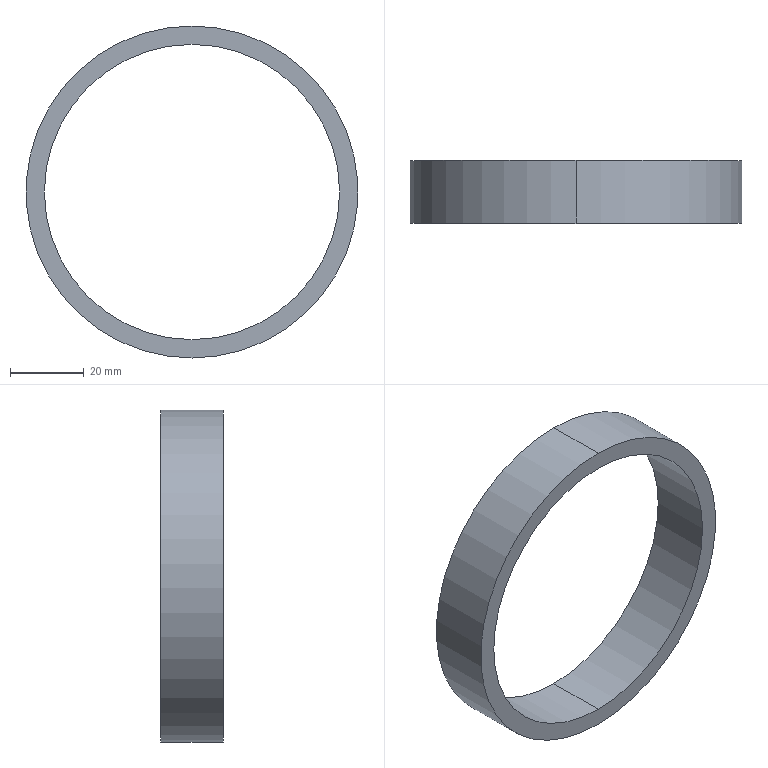Part | NX | features BREP 1 | 1 solid | 6 faces | box 90 x 17 x 90 mm | volume 22698 mm3 | cylinder 4 | plane 2 | commonest cylinder face diameters 80 x2 90 x2
STEP:
#1=CARTESIAN_POINT('',(0.,17.,-40.));
#2=VERTEX_POINT('',#1);
#3=CARTESIAN_POINT('',(0.,17.,40.));
#4=VERTEX_POINT('',#3);
#5=CARTESIAN_POINT('',(0.,17.,0.));
#6=DIRECTION('',(0.,1.,0.));
#7=DIRECTION('',(0.,0.,1.));
#8=AXIS2_PLACEMENT_3D('',#5,#6,#7);
#9=CIRCLE('',#8,40.);
#10=EDGE_CURVE('',#2,#4,#9,.T.);
#11=ORIENTED_EDGE('',*,*,#10,.T.);
#12=CARTESIAN_POINT('',(0.,0.,40.));
#13=VERTEX_POINT('',#12);
#14=CARTESIAN_POINT('',(0.,17.,40.));
#15=DIRECTION('',(0.,-1.,0.));
#16=VECTOR('',#15,1000.);
#17=LINE('',#14,#16);
#18=EDGE_CURVE('',#13,#4,#17,.F.);
#19=ORIENTED_EDGE('',*,*,#18,.F.);
#20=CARTESIAN_POINT('',(0.,0.,-40.));
#21=VERTEX_POINT('',#20);
#22=CARTESIAN_POINT('',(0.,0.,0.));
#23=DIRECTION('',(0.,1.,0.));
#24=DIRECTION('',(0.,0.,1.));
#25=AXIS2_PLACEMENT_3D('',#22,#23,#24);
#26=CIRCLE('',#25,40.);
#27=EDGE_CURVE('',#21,#13,#26,.T.);
#28=ORIENTED_EDGE('',*,*,#27,.F.);
#29=CARTESIAN_POINT('',(0.,17.,-40.));
#30=DIRECTION('',(0.,-1.,0.));
#31=VECTOR('',#30,1000.);
#32=LINE('',#29,#31);
#33=EDGE_CURVE('',#21,#2,#32,.F.);
#34=ORIENTED_EDGE('',*,*,#33,.T.);
#35=EDGE_LOOP('',(#11,#19,#28,#34));
#36=FACE_BOUND('',#35,.T.);
#37=CARTESIAN_POINT('',(0.,17.,0.));
#38=DIRECTION('',(0.,-1.,0.));
#39=DIRECTION('',(0.,0.,1.));
#40=AXIS2_PLACEMENT_3D('',#37,#38,#39);
#41=CYLINDRICAL_SURFACE('',#40,40.);
#42=ADVANCED_FACE('',(#36),#41,.F.);
#43=CARTESIAN_POINT('',(0.,17.,45.));
#44=VERTEX_POINT('',#43);
#45=CARTESIAN_POINT('',(0.,17.,-45.));
#46=VERTEX_POINT('',#45);
#47=CARTESIAN_POINT('',(0.,17.,0.));
#48=DIRECTION('',(0.,1.,0.));
#49=DIRECTION('',(0.,0.,1.));
#50=AXIS2_PLACEMENT_3D('',#47,#48,#49);
#51=CIRCLE('',#50,45.);
#52=EDGE_CURVE('',#44,#46,#51,.T.);
#53=ORIENTED_EDGE('',*,*,#52,.F.);
#54=CARTESIAN_POINT('',(0.,0.,45.));
#55=VERTEX_POINT('',#54);
#56=CARTESIAN_POINT('',(0.,17.,45.));
#57=DIRECTION('',(0.,-1.,0.));
#58=VECTOR('',#57,1000.);
#59=LINE('',#56,#58);
#60=EDGE_CURVE('',#55,#44,#59,.F.);
#61=ORIENTED_EDGE('',*,*,#60,.F.);
#62=CARTESIAN_POINT('',(0.,0.,-45.));
#63=VERTEX_POINT('',#62);
#64=CARTESIAN_POINT('',(0.,0.,0.));
#65=DIRECTION('',(0.,1.,0.));
#66=DIRECTION('',(0.,0.,1.));
#67=AXIS2_PLACEMENT_3D('',#64,#65,#66);
#68=CIRCLE('',#67,45.);
#69=EDGE_CURVE('',#55,#63,#68,.T.);
#70=ORIENTED_EDGE('',*,*,#69,.T.);
#71=CARTESIAN_POINT('',(0.,17.,-45.));
#72=DIRECTION('',(0.,-1.,0.));
#73=VECTOR('',#72,1000.);
#74=LINE('',#71,#73);
#75=EDGE_CURVE('',#63,#46,#74,.F.);
#76=ORIENTED_EDGE('',*,*,#75,.T.);
#77=EDGE_LOOP('',(#53,#61,#70,#76));
#78=FACE_BOUND('',#77,.T.);
#79=CARTESIAN_POINT('',(0.,17.,0.));
#80=DIRECTION('',(0.,-1.,0.));
#81=DIRECTION('',(0.,0.,1.));
#82=AXIS2_PLACEMENT_3D('',#79,#80,#81);
#83=CYLINDRICAL_SURFACE('',#82,45.);
#84=ADVANCED_FACE('',(#78),#83,.T.);
#85=CARTESIAN_POINT('',(0.,17.,0.));
#86=DIRECTION('',(0.,1.,0.));
#87=DIRECTION('',(0.,0.,1.));
#88=AXIS2_PLACEMENT_3D('',#85,#86,#87);
#89=CIRCLE('',#88,45.);
#90=EDGE_CURVE('',#46,#44,#89,.T.);
#91=ORIENTED_EDGE('',*,*,#90,.T.);
#92=ORIENTED_EDGE('',*,*,#52,.T.);
#93=EDGE_LOOP('',(#91,#92));
#94=FACE_BOUND('',#93,.T.);
#95=ORIENTED_EDGE('',*,*,#10,.F.);
#96=CARTESIAN_POINT('',(0.,17.,0.));
#97=DIRECTION('',(0.,1.,0.));
#98=DIRECTION('',(0.,0.,1.));
#99=AXIS2_PLACEMENT_3D('',#96,#97,#98);
#100=CIRCLE('',#99,40.);
#101=EDGE_CURVE('',#4,#2,#100,.T.);
#102=ORIENTED_EDGE('',*,*,#101,.F.);
#103=EDGE_LOOP('',(#95,#102));
#104=FACE_BOUND('',#103,.T.);
#105=CARTESIAN_POINT('',(0.,17.,0.));
#106=DIRECTION('',(0.,1.,0.));
#107=DIRECTION('',(0.,0.,1.));
#108=AXIS2_PLACEMENT_3D('',#105,#106,#107);
#109=PLANE('',#108);
#110=ADVANCED_FACE('',(#94,#104),#109,.T.);
#111=CARTESIAN_POINT('',(0.,0.,0.));
#112=DIRECTION('',(0.,1.,0.));
#113=DIRECTION('',(0.,0.,1.));
#114=AXIS2_PLACEMENT_3D('',#111,#112,#113);
#115=CIRCLE('',#114,45.);
#116=EDGE_CURVE('',#63,#55,#115,.T.);
#117=ORIENTED_EDGE('',*,*,#116,.F.);
#118=ORIENTED_EDGE('',*,*,#69,.F.);
#119=EDGE_LOOP('',(#117,#118));
#120=FACE_BOUND('',#119,.T.);
#121=ORIENTED_EDGE('',*,*,#27,.T.);
#122=CARTESIAN_POINT('',(0.,0.,0.));
#123=DIRECTION('',(0.,1.,0.));
#124=DIRECTION('',(0.,0.,1.));
#125=AXIS2_PLACEMENT_3D('',#122,#123,#124);
#126=CIRCLE('',#125,40.);
#127=EDGE_CURVE('',#13,#21,#126,.T.);
#128=ORIENTED_EDGE('',*,*,#127,.T.);
#129=EDGE_LOOP('',(#121,#128));
#130=FACE_BOUND('',#129,.T.);
#131=CARTESIAN_POINT('',(0.,0.,0.));
#132=DIRECTION('',(0.,1.,0.));
#133=DIRECTION('',(0.,0.,1.));
#134=AXIS2_PLACEMENT_3D('',#131,#132,#133);
#135=PLANE('',#134);
#136=ADVANCED_FACE('',(#120,#130),#135,.F.);
#137=ORIENTED_EDGE('',*,*,#60,.T.);
#138=ORIENTED_EDGE('',*,*,#90,.F.);
#139=ORIENTED_EDGE('',*,*,#75,.F.);
#140=ORIENTED_EDGE('',*,*,#116,.T.);
#141=EDGE_LOOP('',(#137,#138,#139,#140));
#142=FACE_BOUND('',#141,.T.);
#143=CARTESIAN_POINT('',(0.,17.,0.));
#144=DIRECTION('',(0.,-1.,0.));
#145=DIRECTION('',(0.,0.,1.));
#146=AXIS2_PLACEMENT_3D('',#143,#144,#145);
#147=CYLINDRICAL_SURFACE('',#146,45.);
#148=ADVANCED_FACE('',(#142),#147,.T.);
#149=ORIENTED_EDGE('',*,*,#18,.T.);
#150=ORIENTED_EDGE('',*,*,#101,.T.);
#151=ORIENTED_EDGE('',*,*,#33,.F.);
#152=ORIENTED_EDGE('',*,*,#127,.F.);
#153=EDGE_LOOP('',(#149,#150,#151,#152));
#154=FACE_BOUND('',#153,.T.);
#155=CARTESIAN_POINT('',(0.,17.,0.));
#156=DIRECTION('',(0.,-1.,0.));
#157=DIRECTION('',(0.,0.,1.));
#158=AXIS2_PLACEMENT_3D('',#155,#156,#157);
#159=CYLINDRICAL_SURFACE('',#158,40.);
#160=ADVANCED_FACE('',(#154),#159,.F.);
#161=CLOSED_SHELL('',(#42,#84,#110,#136,#148,#160));
#162=MANIFOLD_SOLID_BREP('',#161);
#163=(LENGTH_UNIT()NAMED_UNIT(*)SI_UNIT(.MILLI.,.METRE.));
#164=UNCERTAINTY_MEASURE_WITH_UNIT(LENGTH_MEASURE(0.00001),#163,'','');
#165=(NAMED_UNIT(*)PLANE_ANGLE_UNIT()SI_UNIT($,.RADIAN.));
#166=(NAMED_UNIT(*)SI_UNIT($,.STERADIAN.)SOLID_ANGLE_UNIT());
#167=(GEOMETRIC_REPRESENTATION_CONTEXT(3)GLOBAL_UNCERTAINTY_ASSIGNED_CONTEXT((#164))GLOBAL_UNIT_ASSIGNED_CONTEXT((#163,#165,#166))REPRESENTATION_CONTEXT('',''));
#168=ADVANCED_BREP_SHAPE_REPRESENTATION('',(#162),#167);